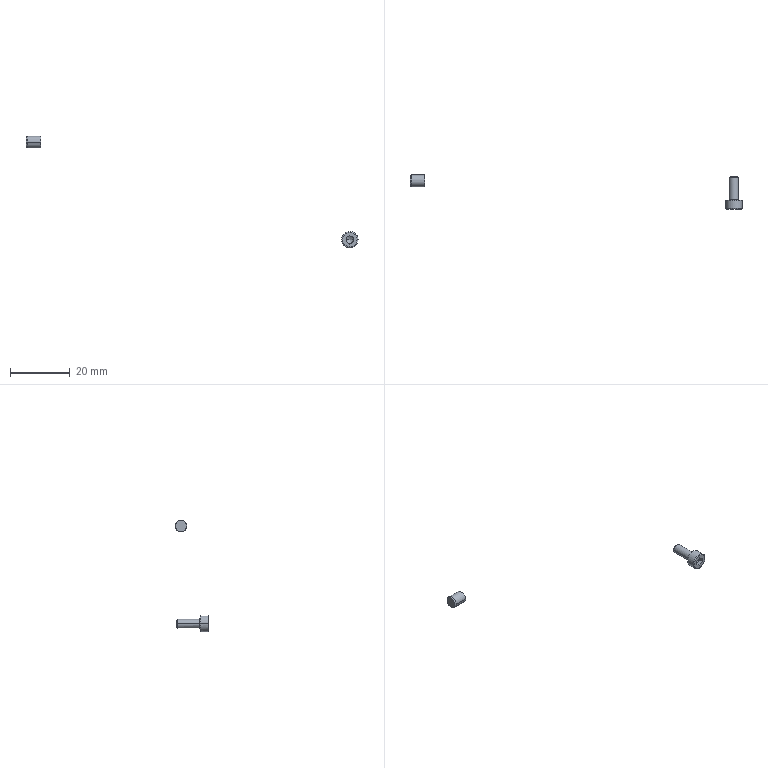Part | STEP file | ASND-0110-IRB120_3-58_IRC5_Link4_rev0-1 | 2 solids | 33 faces | box 111.545 x 11.377 x 37.543 mm | volume 181.054 mm3 | plane 17 | cone 6 | cylinder 6 | torus 4 | commonest cylinder face diameters 3 x2 4 x2 5.5 x2